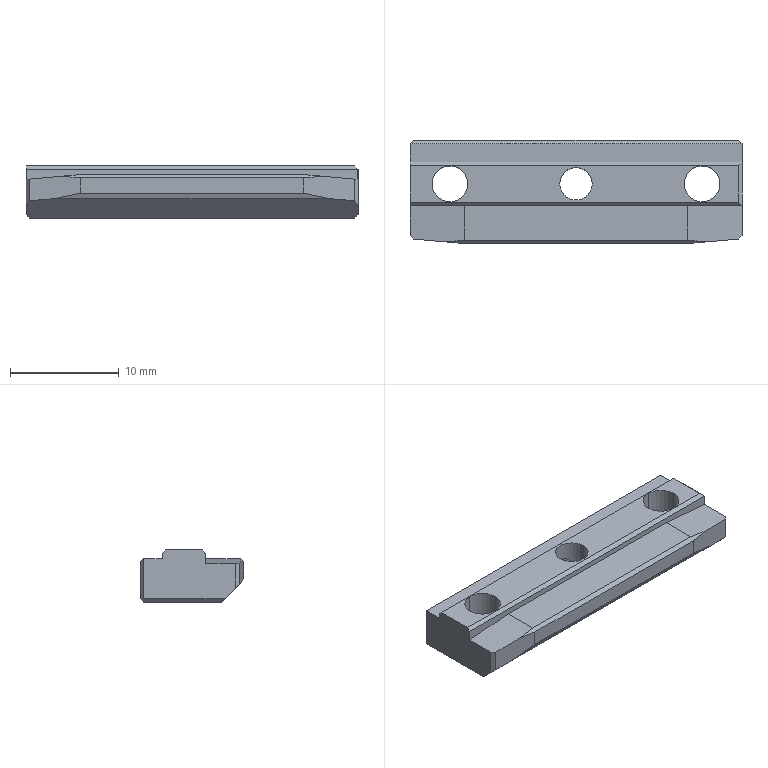Part | NX | 1 solid | 43 faces | box 30.6 x 9.5 x 4.8 mm | volume 1049 mm3 | plane 29 | cylinder 8 | cone 6 | commonest cylinder face diameters 3.3 x4 2.5 x2 3 x2